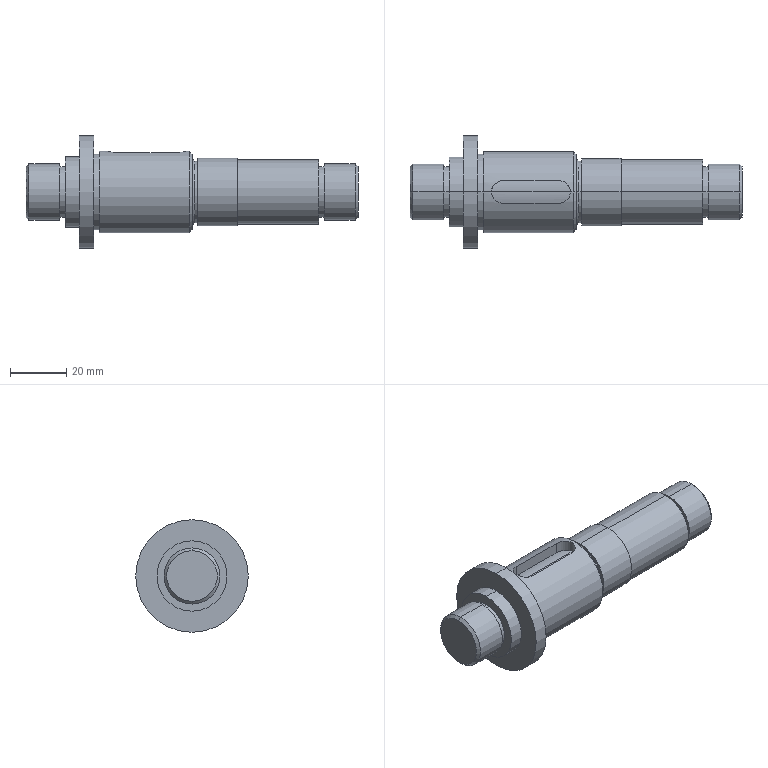Part | SolidWorks | features ICE 11, Chamfer 1, Extrusion 1 | 1 solid | 48 faces | box 118 x 40 x 40 mm | volume 58470 mm3 | cylinder 24 | plane 14 | cone 8 | spline 2 | commonest cylinder face diameters 18 x4 20 x4 29 x4 22 x2 23 x2 24 x2
STEP:
#1=CARTESIAN_POINT('',(0.,0.,9.));
#2=VERTEX_POINT('',#1);
#3=CARTESIAN_POINT('',(0.,0.,-9.));
#4=VERTEX_POINT('',#3);
#5=CARTESIAN_POINT('',(0.,0.,0.));
#6=DIRECTION('',(-1.,0.,0.));
#7=DIRECTION('',(0.,0.,-1.));
#8=AXIS2_PLACEMENT_3D('',#5,#6,#7);
#9=CIRCLE('',#8,9.);
#10=EDGE_CURVE('',#2,#4,#9,.T.);
#11=ORIENTED_EDGE('',*,*,#10,.F.);
#12=CARTESIAN_POINT('',(1.,0.,10.));
#13=VERTEX_POINT('',#12);
#14=CARTESIAN_POINT('',(1.,0.,10.));
#15=DIRECTION('',(0.7071,0.,0.7071));
#16=VECTOR('',#15,1000.);
#17=LINE('',#14,#16);
#18=EDGE_CURVE('',#2,#13,#17,.T.);
#19=ORIENTED_EDGE('',*,*,#18,.T.);
#20=CARTESIAN_POINT('',(1.,0.,-10.));
#21=VERTEX_POINT('',#20);
#22=CARTESIAN_POINT('',(1.,0.,0.));
#23=DIRECTION('',(1.,0.,0.));
#24=DIRECTION('',(0.,0.,-1.));
#25=AXIS2_PLACEMENT_3D('',#22,#23,#24);
#26=CIRCLE('',#25,10.);
#27=EDGE_CURVE('',#21,#13,#26,.T.);
#28=ORIENTED_EDGE('',*,*,#27,.F.);
#29=CARTESIAN_POINT('',(1.,0.,-10.));
#30=DIRECTION('',(0.7071,0.,-0.7071));
#31=VECTOR('',#30,1000.);
#32=LINE('',#29,#31);
#33=EDGE_CURVE('',#4,#21,#32,.T.);
#34=ORIENTED_EDGE('',*,*,#33,.F.);
#35=EDGE_LOOP('',(#11,#19,#28,#34));
#36=FACE_OUTER_BOUND('',#35,.T.);
#37=CARTESIAN_POINT('',(1.,0.,0.));
#38=DIRECTION('',(1.,0.,0.));
#39=DIRECTION('',(0.,0.,-1.));
#40=AXIS2_PLACEMENT_3D('',#37,#38,#39);
#41=CONICAL_SURFACE('',#40,10.,0.7854);
#42=ADVANCED_FACE('',(#36),#41,.T.);
#43=CARTESIAN_POINT('',(118.,0.,-9.));
#44=VERTEX_POINT('',#43);
#45=CARTESIAN_POINT('',(118.,0.,9.));
#46=VERTEX_POINT('',#45);
#47=CARTESIAN_POINT('',(118.,0.,0.));
#48=DIRECTION('',(1.,0.,0.));
#49=DIRECTION('',(0.,0.,-1.));
#50=AXIS2_PLACEMENT_3D('',#47,#48,#49);
#51=CIRCLE('',#50,9.);
#52=EDGE_CURVE('',#44,#46,#51,.T.);
#53=ORIENTED_EDGE('',*,*,#52,.F.);
#54=CARTESIAN_POINT('',(117.,0.,-10.));
#55=VERTEX_POINT('',#54);
#56=CARTESIAN_POINT('',(118.,0.,-9.));
#57=DIRECTION('',(-0.7071,0.,-0.7071));
#58=VECTOR('',#57,1000.);
#59=LINE('',#56,#58);
#60=EDGE_CURVE('',#44,#55,#59,.T.);
#61=ORIENTED_EDGE('',*,*,#60,.T.);
#62=CARTESIAN_POINT('',(117.,0.,10.));
#63=VERTEX_POINT('',#62);
#64=CARTESIAN_POINT('',(117.,0.,0.));
#65=DIRECTION('',(-1.,0.,0.));
#66=DIRECTION('',(0.,0.,-1.));
#67=AXIS2_PLACEMENT_3D('',#64,#65,#66);
#68=CIRCLE('',#67,10.);
#69=EDGE_CURVE('',#63,#55,#68,.T.);
#70=ORIENTED_EDGE('',*,*,#69,.F.);
#71=CARTESIAN_POINT('',(118.,0.,9.));
#72=DIRECTION('',(-0.7071,0.,0.7071));
#73=VECTOR('',#72,1000.);
#74=LINE('',#71,#73);
#75=EDGE_CURVE('',#46,#63,#74,.T.);
#76=ORIENTED_EDGE('',*,*,#75,.F.);
#77=EDGE_LOOP('',(#53,#61,#70,#76));
#78=FACE_OUTER_BOUND('',#77,.T.);
#79=CARTESIAN_POINT('',(118.,0.,0.));
#80=DIRECTION('',(-1.,0.,0.));
#81=DIRECTION('',(0.,0.,1.));
#82=AXIS2_PLACEMENT_3D('',#79,#80,#81);
#83=CONICAL_SURFACE('',#82,9.,0.7854);
#84=ADVANCED_FACE('',(#78),#83,.T.);
#85=CARTESIAN_POINT('',(60.,0.,-11.));
#86=VERTEX_POINT('',#85);
#87=CARTESIAN_POINT('',(60.,0.,11.));
#88=VERTEX_POINT('',#87);
#89=CARTESIAN_POINT('',(60.,0.,0.));
#90=DIRECTION('',(1.,0.,0.));
#91=DIRECTION('',(0.,0.,-1.));
#92=AXIS2_PLACEMENT_3D('',#89,#90,#91);
#93=CIRCLE('',#92,11.);
#94=EDGE_CURVE('',#86,#88,#93,.T.);
#95=ORIENTED_EDGE('',*,*,#94,.F.);
#96=CARTESIAN_POINT('',(59.,0.,-12.));
#97=VERTEX_POINT('',#96);
#98=CARTESIAN_POINT('',(60.,0.,-11.));
#99=DIRECTION('',(-0.7071,0.,-0.7071));
#100=VECTOR('',#99,1000.);
#101=LINE('',#98,#100);
#102=EDGE_CURVE('',#86,#97,#101,.T.);
#103=ORIENTED_EDGE('',*,*,#102,.T.);
#104=CARTESIAN_POINT('',(59.,0.,12.));
#105=VERTEX_POINT('',#104);
#106=CARTESIAN_POINT('',(59.,0.,0.));
#107=DIRECTION('',(-1.,0.,0.));
#108=DIRECTION('',(0.,0.,-1.));
#109=AXIS2_PLACEMENT_3D('',#106,#107,#108);
#110=CIRCLE('',#109,12.);
#111=EDGE_CURVE('',#105,#97,#110,.T.);
#112=ORIENTED_EDGE('',*,*,#111,.F.);
#113=CARTESIAN_POINT('',(60.,0.,11.));
#114=DIRECTION('',(-0.7071,0.,0.7071));
#115=VECTOR('',#114,1000.);
#116=LINE('',#113,#115);
#117=EDGE_CURVE('',#88,#105,#116,.T.);
#118=ORIENTED_EDGE('',*,*,#117,.F.);
#119=EDGE_LOOP('',(#95,#103,#112,#118));
#120=FACE_OUTER_BOUND('',#119,.T.);
#121=CARTESIAN_POINT('',(60.,0.,0.));
#122=DIRECTION('',(-1.,0.,0.));
#123=DIRECTION('',(0.,0.,1.));
#124=AXIS2_PLACEMENT_3D('',#121,#122,#123);
#125=CONICAL_SURFACE('',#124,11.,0.7854);
#126=ADVANCED_FACE('',(#120),#125,.T.);
#127=CARTESIAN_POINT('',(59.,0.,-13.5));
#128=VERTEX_POINT('',#127);
#129=CARTESIAN_POINT('',(59.,0.,13.5));
#130=VERTEX_POINT('',#129);
#131=CARTESIAN_POINT('',(59.,0.,0.));
#132=DIRECTION('',(1.,0.,0.));
#133=DIRECTION('',(0.,0.,-1.));
#134=AXIS2_PLACEMENT_3D('',#131,#132,#133);
#135=CIRCLE('',#134,13.5);
#136=EDGE_CURVE('',#128,#130,#135,.T.);
#137=ORIENTED_EDGE('',*,*,#136,.F.);
#138=CARTESIAN_POINT('',(58.,0.,-14.5));
#139=VERTEX_POINT('',#138);
#140=CARTESIAN_POINT('',(59.,0.,-13.5));
#141=DIRECTION('',(-0.7071,0.,-0.7071));
#142=VECTOR('',#141,1000.);
#143=LINE('',#140,#142);
#144=EDGE_CURVE('',#128,#139,#143,.T.);
#145=ORIENTED_EDGE('',*,*,#144,.T.);
#146=CARTESIAN_POINT('',(58.,0.,14.5));
#147=VERTEX_POINT('',#146);
#148=CARTESIAN_POINT('',(58.,0.,0.));
#149=DIRECTION('',(-1.,0.,0.));
#150=DIRECTION('',(0.,0.,-1.));
#151=AXIS2_PLACEMENT_3D('',#148,#149,#150);
#152=CIRCLE('',#151,14.5);
#153=EDGE_CURVE('',#147,#139,#152,.T.);
#154=ORIENTED_EDGE('',*,*,#153,.F.);
#155=CARTESIAN_POINT('',(59.,0.,13.5));
#156=DIRECTION('',(-0.7071,0.,0.7071));
#157=VECTOR('',#156,1000.);
#158=LINE('',#155,#157);
#159=EDGE_CURVE('',#130,#147,#158,.T.);
#160=ORIENTED_EDGE('',*,*,#159,.F.);
#161=EDGE_LOOP('',(#137,#145,#154,#160));
#162=FACE_OUTER_BOUND('',#161,.T.);
#163=CARTESIAN_POINT('',(59.,0.,0.));
#164=DIRECTION('',(-1.,0.,0.));
#165=DIRECTION('',(0.,0.,1.));
#166=AXIS2_PLACEMENT_3D('',#163,#164,#165);
#167=CONICAL_SURFACE('',#166,13.5,0.7854);
#168=ADVANCED_FACE('',(#162),#167,.T.);
#169=CARTESIAN_POINT('',(53.,-4.,9.937));
#170=VERTEX_POINT('',#169);
#171=CARTESIAN_POINT('',(57.,0.000000128,10.5));
#172=VERTEX_POINT('',#171);
#173=CARTESIAN_POINT('',(53.,-4.,9.937));
#174=CARTESIAN_POINT('',(53.264,-4.,9.937));
#175=CARTESIAN_POINT('',(53.531,-3.972,9.945));
#176=CARTESIAN_POINT('',(54.044,-3.867,9.975));
#177=CARTESIAN_POINT('',(54.297,-3.789,9.997));
#178=CARTESIAN_POINT('',(55.02,-3.488,10.076));
#179=CARTESIAN_POINT('',(55.464,-3.193,10.149));
#180=CARTESIAN_POINT('',(56.012,-2.644,10.258));
#181=CARTESIAN_POINT('',(56.178,-2.441,10.295));
#182=CARTESIAN_POINT('',(56.466,-2.006,10.362));
#183=CARTESIAN_POINT('',(56.589,-1.775,10.393));
#184=CARTESIAN_POINT('',(56.791,-1.29,10.445));
#185=CARTESIAN_POINT('',(56.868,-1.04,10.465));
#186=CARTESIAN_POINT('',(56.973,-0.5231,10.493));
#187=CARTESIAN_POINT('',(57.,-0.2611,10.5));
#188=CARTESIAN_POINT('',(57.,0.000000128,10.5));
#189=B_SPLINE_CURVE_WITH_KNOTS('',3,(#173,#174,#175,#176,#177,#178,#179,#180,#181,#182,#183,#184,#185,#186,#187,#188),.UNSPECIFIED.,.F.,.F.,(4,2,2,2,2,2,2,4),(0.,0.06254,0.1251,0.2501,0.3127,0.3752,0.4378,0.5003),.UNSPECIFIED.);
#190=EDGE_CURVE('',#170,#172,#189,.T.);
#191=ORIENTED_EDGE('',*,*,#190,.T.);
#192=CARTESIAN_POINT('',(29.,-0.000000128,10.5));
#193=VERTEX_POINT('',#192);
#194=CARTESIAN_POINT('',(59.,0.,10.5));
#195=DIRECTION('',(-1.,0.,0.));
#196=VECTOR('',#195,1000.);
#197=LINE('',#194,#196);
#198=EDGE_CURVE('',#172,#193,#197,.T.);
#199=ORIENTED_EDGE('',*,*,#198,.T.);
#200=CARTESIAN_POINT('',(33.,-4.,9.937));
#201=VERTEX_POINT('',#200);
#202=CARTESIAN_POINT('',(29.,-0.000000128,10.5));
#203=CARTESIAN_POINT('',(29.,-0.2608,10.5));
#204=CARTESIAN_POINT('',(29.027,-0.5243,10.493));
#205=CARTESIAN_POINT('',(29.131,-1.037,10.465));
#206=CARTESIAN_POINT('',(29.208,-1.288,10.445));
#207=CARTESIAN_POINT('',(29.509,-2.015,10.368));
#208=CARTESIAN_POINT('',(29.803,-2.46,10.295));
#209=CARTESIAN_POINT('',(30.356,-3.013,10.185));
#210=CARTESIAN_POINT('',(30.559,-3.179,10.148));
#211=CARTESIAN_POINT('',(30.993,-3.468,10.08));
#212=CARTESIAN_POINT('',(31.223,-3.591,10.049));
#213=CARTESIAN_POINT('',(31.707,-3.792,9.996));
#214=CARTESIAN_POINT('',(31.955,-3.868,9.975));
#215=CARTESIAN_POINT('',(32.343,-3.947,9.953));
#216=CARTESIAN_POINT('',(32.472,-3.966,9.947));
#217=CARTESIAN_POINT('',(32.736,-3.993,9.939));
#218=CARTESIAN_POINT('',(32.868,-4.,9.937));
#219=CARTESIAN_POINT('',(33.,-4.,9.937));
#220=B_SPLINE_CURVE_WITH_KNOTS('',3,(#202,#203,#204,#205,#206,#207,#208,#209,#210,#211,#212,#213,#214,#215,#216,#217,#218,#219),.UNSPECIFIED.,.F.,.F.,(4,2,2,2,2,2,2,2,4),(0.5003,0.5628,0.6252,0.7501,0.8126,0.8751,0.9375,0.9688,1.),.UNSPECIFIED.);
#221=EDGE_CURVE('',#193,#201,#220,.T.);
#222=ORIENTED_EDGE('',*,*,#221,.T.);
#223=CARTESIAN_POINT('',(59.,-4.,9.937));
#224=DIRECTION('',(-1.,0.,0.));
#225=VECTOR('',#224,1000.);
#226=LINE('',#223,#225);
#227=EDGE_CURVE('',#170,#201,#226,.T.);
#228=ORIENTED_EDGE('',*,*,#227,.F.);
#229=EDGE_LOOP('',(#191,#199,#222,#228));
#230=FACE_OUTER_BOUND('',#229,.T.);
#231=CARTESIAN_POINT('',(59.,0.,-4.));
#232=DIRECTION('',(-1.,0.,0.));
#233=DIRECTION('',(0.,0.,1.));
#234=AXIS2_PLACEMENT_3D('',#231,#232,#233);
#235=CYLINDRICAL_SURFACE('',#234,14.5);
#236=ADVANCED_FACE('',(#230),#235,.T.);
#237=ORIENTED_EDGE('',*,*,#69,.T.);
#238=CARTESIAN_POINT('',(106.,0.,-10.));
#239=VERTEX_POINT('',#238);
#240=CARTESIAN_POINT('',(118.,0.,-10.));
#241=DIRECTION('',(-1.,0.,0.));
#242=VECTOR('',#241,1000.);
#243=LINE('',#240,#242);
#244=EDGE_CURVE('',#55,#239,#243,.T.);
#245=ORIENTED_EDGE('',*,*,#244,.T.);
#246=CARTESIAN_POINT('',(106.,0.,10.));
#247=VERTEX_POINT('',#246);
#248=CARTESIAN_POINT('',(106.,0.,0.));
#249=DIRECTION('',(1.,0.,0.));
#250=DIRECTION('',(0.,0.,-1.));
#251=AXIS2_PLACEMENT_3D('',#248,#249,#250);
#252=CIRCLE('',#251,10.);
#253=EDGE_CURVE('',#239,#247,#252,.T.);
#254=ORIENTED_EDGE('',*,*,#253,.T.);
#255=CARTESIAN_POINT('',(118.,0.,10.));
#256=DIRECTION('',(-1.,0.,0.));
#257=VECTOR('',#256,1000.);
#258=LINE('',#255,#257);
#259=EDGE_CURVE('',#63,#247,#258,.T.);
#260=ORIENTED_EDGE('',*,*,#259,.F.);
#261=EDGE_LOOP('',(#237,#245,#254,#260));
#262=FACE_OUTER_BOUND('',#261,.T.);
#263=CARTESIAN_POINT('',(118.,0.,0.));
#264=DIRECTION('',(-1.,0.,0.));
#265=DIRECTION('',(0.,0.,1.));
#266=AXIS2_PLACEMENT_3D('',#263,#264,#265);
#267=CYLINDRICAL_SURFACE('',#266,10.);
#268=ADVANCED_FACE('',(#262),#267,.T.);
#269=CARTESIAN_POINT('',(106.,0.,-9.));
#270=VERTEX_POINT('',#269);
#271=CARTESIAN_POINT('',(106.,0.,9.));
#272=VERTEX_POINT('',#271);
#273=CARTESIAN_POINT('',(106.,0.,0.));
#274=DIRECTION('',(1.,0.,0.));
#275=DIRECTION('',(0.,0.,-1.));
#276=AXIS2_PLACEMENT_3D('',#273,#274,#275);
#277=CIRCLE('',#276,9.);
#278=EDGE_CURVE('',#270,#272,#277,.T.);
#279=ORIENTED_EDGE('',*,*,#278,.F.);
#280=CARTESIAN_POINT('',(104.,0.,-9.));
#281=VERTEX_POINT('',#280);
#282=CARTESIAN_POINT('',(106.,0.,-9.));
#283=DIRECTION('',(-1.,0.,0.));
#284=VECTOR('',#283,1000.);
#285=LINE('',#282,#284);
#286=EDGE_CURVE('',#270,#281,#285,.T.);
#287=ORIENTED_EDGE('',*,*,#286,.T.);
#288=CARTESIAN_POINT('',(104.,0.,9.));
#289=VERTEX_POINT('',#288);
#290=CARTESIAN_POINT('',(104.,0.,0.));
#291=DIRECTION('',(1.,0.,0.));
#292=DIRECTION('',(0.,0.,-1.));
#293=AXIS2_PLACEMENT_3D('',#290,#291,#292);
#294=CIRCLE('',#293,9.);
#295=EDGE_CURVE('',#281,#289,#294,.T.);
#296=ORIENTED_EDGE('',*,*,#295,.T.);
#297=CARTESIAN_POINT('',(106.,0.,9.));
#298=DIRECTION('',(-1.,0.,0.));
#299=VECTOR('',#298,1000.);
#300=LINE('',#297,#299);
#301=EDGE_CURVE('',#272,#289,#300,.T.);
#302=ORIENTED_EDGE('',*,*,#301,.F.);
#303=EDGE_LOOP('',(#279,#287,#296,#302));
#304=FACE_OUTER_BOUND('',#303,.T.);
#305=CARTESIAN_POINT('',(106.,0.,0.));
#306=DIRECTION('',(-1.,0.,0.));
#307=DIRECTION('',(0.,0.,1.));
#308=AXIS2_PLACEMENT_3D('',#305,#306,#307);
#309=CYLINDRICAL_SURFACE('',#308,9.);
#310=ADVANCED_FACE('',(#304),#309,.T.);
#311=CARTESIAN_POINT('',(104.,0.,-11.5));
#312=VERTEX_POINT('',#311);
#313=CARTESIAN_POINT('',(104.,0.,11.5));
#314=VERTEX_POINT('',#313);
#315=CARTESIAN_POINT('',(104.,0.,0.));
#316=DIRECTION('',(1.,0.,0.));
#317=DIRECTION('',(0.,0.,-1.));
#318=AXIS2_PLACEMENT_3D('',#315,#316,#317);
#319=CIRCLE('',#318,11.5);
#320=EDGE_CURVE('',#312,#314,#319,.T.);
#321=ORIENTED_EDGE('',*,*,#320,.F.);
#322=CARTESIAN_POINT('',(75.,0.,-11.5));
#323=VERTEX_POINT('',#322);
#324=CARTESIAN_POINT('',(104.,0.,-11.5));
#325=DIRECTION('',(-1.,0.,0.));
#326=VECTOR('',#325,1000.);
#327=LINE('',#324,#326);
#328=EDGE_CURVE('',#312,#323,#327,.T.);
#329=ORIENTED_EDGE('',*,*,#328,.T.);
#330=CARTESIAN_POINT('',(75.,0.,11.5));
#331=VERTEX_POINT('',#330);
#332=CARTESIAN_POINT('',(75.,0.,0.));
#333=DIRECTION('',(1.,0.,0.));
#334=DIRECTION('',(0.,0.,-1.));
#335=AXIS2_PLACEMENT_3D('',#332,#333,#334);
#336=CIRCLE('',#335,11.5);
#337=EDGE_CURVE('',#323,#331,#336,.T.);
#338=ORIENTED_EDGE('',*,*,#337,.T.);
#339=CARTESIAN_POINT('',(104.,0.,11.5));
#340=DIRECTION('',(-1.,0.,0.));
#341=VECTOR('',#340,1000.);
#342=LINE('',#339,#341);
#343=EDGE_CURVE('',#314,#331,#342,.T.);
#344=ORIENTED_EDGE('',*,*,#343,.F.);
#345=EDGE_LOOP('',(#321,#329,#338,#344));
#346=FACE_OUTER_BOUND('',#345,.T.);
#347=CARTESIAN_POINT('',(104.,0.,0.));
#348=DIRECTION('',(-1.,0.,0.));
#349=DIRECTION('',(0.,0.,1.));
#350=AXIS2_PLACEMENT_3D('',#347,#348,#349);
#351=CYLINDRICAL_SURFACE('',#350,11.5);
#352=ADVANCED_FACE('',(#346),#351,.T.);
#353=CARTESIAN_POINT('',(75.,0.,-12.));
#354=VERTEX_POINT('',#353);
#355=CARTESIAN_POINT('',(75.,0.,12.));
#356=VERTEX_POINT('',#355);
#357=CARTESIAN_POINT('',(75.,0.,0.));
#358=DIRECTION('',(1.,0.,0.));
#359=DIRECTION('',(0.,0.,-1.));
#360=AXIS2_PLACEMENT_3D('',#357,#358,#359);
#361=CIRCLE('',#360,12.);
#362=EDGE_CURVE('',#354,#356,#361,.T.);
#363=ORIENTED_EDGE('',*,*,#362,.F.);
#364=CARTESIAN_POINT('',(61.,0.,-12.));
#365=VERTEX_POINT('',#364);
#366=CARTESIAN_POINT('',(75.,0.,-12.));
#367=DIRECTION('',(-1.,0.,0.));
#368=VECTOR('',#367,1000.);
#369=LINE('',#366,#368);
#370=EDGE_CURVE('',#354,#365,#369,.T.);
#371=ORIENTED_EDGE('',*,*,#370,.T.);
#372=CARTESIAN_POINT('',(61.,0.,12.));
#373=VERTEX_POINT('',#372);
#374=CARTESIAN_POINT('',(61.,0.,0.));
#375=DIRECTION('',(1.,0.,0.));
#376=DIRECTION('',(0.,0.,-1.));
#377=AXIS2_PLACEMENT_3D('',#374,#375,#376);
#378=CIRCLE('',#377,12.);
#379=EDGE_CURVE('',#365,#373,#378,.T.);
#380=ORIENTED_EDGE('',*,*,#379,.T.);
#381=CARTESIAN_POINT('',(75.,0.,12.));
#382=DIRECTION('',(-1.,0.,0.));
#383=VECTOR('',#382,1000.);
#384=LINE('',#381,#383);
#385=EDGE_CURVE('',#356,#373,#384,.T.);
#386=ORIENTED_EDGE('',*,*,#385,.F.);
#387=EDGE_LOOP('',(#363,#371,#380,#386));
#388=FACE_OUTER_BOUND('',#387,.T.);
#389=CARTESIAN_POINT('',(75.,0.,0.));
#390=DIRECTION('',(-1.,0.,0.));
#391=DIRECTION('',(0.,0.,1.));
#392=AXIS2_PLACEMENT_3D('',#389,#390,#391);
#393=CYLINDRICAL_SURFACE('',#392,12.);
#394=ADVANCED_FACE('',(#388),#393,.T.);
#395=CARTESIAN_POINT('',(61.,0.,-11.));
#396=VERTEX_POINT('',#395);
#397=CARTESIAN_POINT('',(61.,0.,11.));
#398=VERTEX_POINT('',#397);
#399=CARTESIAN_POINT('',(61.,0.,0.));
#400=DIRECTION('',(1.,0.,0.));
#401=DIRECTION('',(0.,0.,-1.));
#402=AXIS2_PLACEMENT_3D('',#399,#400,#401);
#403=CIRCLE('',#402,11.);
#404=EDGE_CURVE('',#396,#398,#403,.T.);
#405=ORIENTED_EDGE('',*,*,#404,.F.);
#406=CARTESIAN_POINT('',(61.,0.,-11.));
#407=DIRECTION('',(-1.,0.,0.));
#408=VECTOR('',#407,1000.);
#409=LINE('',#406,#408);
#410=EDGE_CURVE('',#396,#86,#409,.T.);
#411=ORIENTED_EDGE('',*,*,#410,.T.);
#412=ORIENTED_EDGE('',*,*,#94,.T.);
#413=CARTESIAN_POINT('',(61.,0.,11.));
#414=DIRECTION('',(-1.,0.,0.));
#415=VECTOR('',#414,1000.);
#416=LINE('',#413,#415);
#417=EDGE_CURVE('',#398,#88,#416,.T.);
#418=ORIENTED_EDGE('',*,*,#417,.F.);
#419=EDGE_LOOP('',(#405,#411,#412,#418));
#420=FACE_OUTER_BOUND('',#419,.T.);
#421=CARTESIAN_POINT('',(61.,0.,0.));
#422=DIRECTION('',(-1.,0.,0.));
#423=DIRECTION('',(0.,0.,1.));
#424=AXIS2_PLACEMENT_3D('',#421,#422,#423);
#425=CYLINDRICAL_SURFACE('',#424,11.);
#426=ADVANCED_FACE('',(#420),#425,.T.);
#427=ORIENTED_EDGE('',*,*,#153,.T.);
#428=CARTESIAN_POINT('',(26.,0.,-14.5));
#429=VERTEX_POINT('',#428);
#430=CARTESIAN_POINT('',(59.,0.,-14.5));
#431=DIRECTION('',(-1.,0.,0.));
#432=VECTOR('',#431,1000.);
#433=LINE('',#430,#432);
#434=EDGE_CURVE('',#139,#429,#433,.T.);
#435=ORIENTED_EDGE('',*,*,#434,.T.);
#436=CARTESIAN_POINT('',(26.,0.,14.5));
#437=VERTEX_POINT('',#436);
#438=CARTESIAN_POINT('',(26.,0.,0.));
#439=DIRECTION('',(1.,0.,0.));
#440=DIRECTION('',(0.,0.,-1.));
#441=AXIS2_PLACEMENT_3D('',#438,#439,#440);
#442=CIRCLE('',#441,14.5);
#443=EDGE_CURVE('',#429,#437,#442,.T.);
#444=ORIENTED_EDGE('',*,*,#443,.T.);
#445=CARTESIAN_POINT('',(29.,0.000006792,14.5));
#446=VERTEX_POINT('',#445);
#447=CARTESIAN_POINT('',(59.,0.,14.5));
#448=DIRECTION('',(-1.,0.,0.));
#449=VECTOR('',#448,1000.);
#450=LINE('',#447,#449);
#451=EDGE_CURVE('',#446,#437,#450,.T.);
#452=ORIENTED_EDGE('',*,*,#451,.F.);
#453=CARTESIAN_POINT('',(33.,4.,13.937));
#454=VERTEX_POINT('',#453);
#455=CARTESIAN_POINT('',(33.,4.,13.937));
#456=CARTESIAN_POINT('',(31.938,4.,13.937));
#457=CARTESIAN_POINT('',(30.906,3.562,14.075));
#458=CARTESIAN_POINT('',(29.438,2.095,14.367));
#459=CARTESIAN_POINT('',(29.001,1.053,14.5));
#460=CARTESIAN_POINT('',(29.,0.002502,14.5));
#461=CARTESIAN_POINT('',(29.,0.001255,14.5));
#462=CARTESIAN_POINT('',(29.,0.000006792,14.5));
#463=B_SPLINE_CURVE_WITH_KNOTS('',3,(#455,#456,#457,#458,#459,#460,#461,#462),.UNSPECIFIED.,.F.,.F.,(4,2,2,4),(0.,0.25,0.5,0.5003),.UNSPECIFIED.);
#464=EDGE_CURVE('',#454,#446,#463,.T.);
#465=ORIENTED_EDGE('',*,*,#464,.F.);
#466=CARTESIAN_POINT('',(53.,4.,13.937));
#467=VERTEX_POINT('',#466);
#468=CARTESIAN_POINT('',(59.,4.,13.937));
#469=DIRECTION('',(-1.,0.,0.));
#470=VECTOR('',#469,1000.);
#471=LINE('',#468,#470);
#472=EDGE_CURVE('',#467,#454,#471,.T.);
#473=ORIENTED_EDGE('',*,*,#472,.F.);
#474=CARTESIAN_POINT('',(57.,-0.000006792,14.5));
#475=VERTEX_POINT('',#474);
#476=CARTESIAN_POINT('',(57.,-0.000006792,14.5));
#477=CARTESIAN_POINT('',(57.,1.048,14.5));
#478=CARTESIAN_POINT('',(56.568,2.088,14.369));
#479=CARTESIAN_POINT('',(55.09,3.567,14.075));
#480=CARTESIAN_POINT('',(54.062,4.,13.937));
#481=CARTESIAN_POINT('',(53.,4.,13.937));
#482=B_SPLINE_CURVE_WITH_KNOTS('',3,(#476,#477,#478,#479,#480,#481),.UNSPECIFIED.,.F.,.F.,(4,2,4),(0.5003,0.75,1.),.UNSPECIFIED.);
#483=EDGE_CURVE('',#475,#467,#482,.T.);
#484=ORIENTED_EDGE('',*,*,#483,.F.);
#485=CARTESIAN_POINT('',(59.,0.,14.5));
#486=DIRECTION('',(-1.,0.,0.));
#487=VECTOR('',#486,1000.);
#488=LINE('',#485,#487);
#489=EDGE_CURVE('',#147,#475,#488,.T.);
#490=ORIENTED_EDGE('',*,*,#489,.F.);
#491=EDGE_LOOP('',(#427,#435,#444,#452,#465,#473,#484,#490));
#492=FACE_OUTER_BOUND('',#491,.T.);
#493=CARTESIAN_POINT('',(59.,0.,0.));
#494=DIRECTION('',(-1.,0.,0.));
#495=DIRECTION('',(0.,0.,1.));
#496=AXIS2_PLACEMENT_3D('',#493,#494,#495);
#497=CYLINDRICAL_SURFACE('',#496,14.5);
#498=ADVANCED_FACE('',(#492),#497,.T.);
#499=CARTESIAN_POINT('',(26.,0.,-13.5));
#500=VERTEX_POINT('',#499);
#501=CARTESIAN_POINT('',(26.,0.,13.5));
#502=VERTEX_POINT('',#501);
#503=CARTESIAN_POINT('',(26.,0.,0.));
#504=DIRECTION('',(1.,0.,0.));
#505=DIRECTION('',(0.,0.,-1.));
#506=AXIS2_PLACEMENT_3D('',#503,#504,#505);
#507=CIRCLE('',#506,13.5);
#508=EDGE_CURVE('',#500,#502,#507,.T.);
#509=ORIENTED_EDGE('',*,*,#508,.F.);
#510=CARTESIAN_POINT('',(24.,0.,-13.5));
#511=VERTEX_POINT('',#510);
#512=CARTESIAN_POINT('',(26.,0.,-13.5));
#513=DIRECTION('',(-1.,0.,0.));
#514=VECTOR('',#513,1000.);
#515=LINE('',#512,#514);
#516=EDGE_CURVE('',#500,#511,#515,.T.);
#517=ORIENTED_EDGE('',*,*,#516,.T.);
#518=CARTESIAN_POINT('',(24.,0.,13.5));
#519=VERTEX_POINT('',#518);
#520=CARTESIAN_POINT('',(24.,0.,0.));
#521=DIRECTION('',(1.,0.,0.));
#522=DIRECTION('',(0.,0.,-1.));
#523=AXIS2_PLACEMENT_3D('',#520,#521,#522);
#524=CIRCLE('',#523,13.5);
#525=EDGE_CURVE('',#511,#519,#524,.T.);
#526=ORIENTED_EDGE('',*,*,#525,.T.);
#527=CARTESIAN_POINT('',(26.,0.,13.5));
#528=DIRECTION('',(-1.,0.,0.));
#529=VECTOR('',#528,1000.);
#530=LINE('',#527,#529);
#531=EDGE_CURVE('',#502,#519,#530,.T.);
#532=ORIENTED_EDGE('',*,*,#531,.F.);
#533=EDGE_LOOP('',(#509,#517,#526,#532));
#534=FACE_OUTER_BOUND('',#533,.T.);
#535=CARTESIAN_POINT('',(26.,0.,0.));
#536=DIRECTION('',(-1.,0.,0.));
#537=DIRECTION('',(0.,0.,1.));
#538=AXIS2_PLACEMENT_3D('',#535,#536,#537);
#539=CYLINDRICAL_SURFACE('',#538,13.5);
#540=ADVANCED_FACE('',(#534),#539,.T.);
#541=CARTESIAN_POINT('',(24.,0.,-20.));
#542=VERTEX_POINT('',#541);
#543=CARTESIAN_POINT('',(24.,0.,20.));
#544=VERTEX_POINT('',#543);
#545=CARTESIAN_POINT('',(24.,0.,0.));
#546=DIRECTION('',(1.,0.,0.));
#547=DIRECTION('',(0.,0.,-1.));
#548=AXIS2_PLACEMENT_3D('',#545,#546,#547);
#549=CIRCLE('',#548,20.);
#550=EDGE_CURVE('',#542,#544,#549,.T.);
#551=ORIENTED_EDGE('',*,*,#550,.F.);
#552=CARTESIAN_POINT('',(19.,0.,-20.));
#553=VERTEX_POINT('',#552);
#554=CARTESIAN_POINT('',(24.,0.,-20.));
#555=DIRECTION('',(-1.,0.,0.));
#556=VECTOR('',#555,1000.);
#557=LINE('',#554,#556);
#558=EDGE_CURVE('',#542,#553,#557,.T.);
#559=ORIENTED_EDGE('',*,*,#558,.T.);
#560=CARTESIAN_POINT('',(19.,0.,20.));
#561=VERTEX_POINT('',#560);
#562=CARTESIAN_POINT('',(19.,0.,0.));
#563=DIRECTION('',(1.,0.,0.));
#564=DIRECTION('',(0.,0.,-1.));
#565=AXIS2_PLACEMENT_3D('',#562,#563,#564);
#566=CIRCLE('',#565,20.);
#567=EDGE_CURVE('',#553,#561,#566,.T.);
#568=ORIENTED_EDGE('',*,*,#567,.T.);
#569=CARTESIAN_POINT('',(24.,0.,20.));
#570=DIRECTION('',(-1.,0.,0.));
#571=VECTOR('',#570,1000.);
#572=LINE('',#569,#571);
#573=EDGE_CURVE('',#544,#561,#572,.T.);
#574=ORIENTED_EDGE('',*,*,#573,.F.);
#575=EDGE_LOOP('',(#551,#559,#568,#574));
#576=FACE_OUTER_BOUND('',#575,.T.);
#577=CARTESIAN_POINT('',(24.,0.,0.));
#578=DIRECTION('',(-1.,0.,0.));
#579=DIRECTION('',(0.,0.,1.));
#580=AXIS2_PLACEMENT_3D('',#577,#578,#579);
#581=CYLINDRICAL_SURFACE('',#580,20.);
#582=ADVANCED_FACE('',(#576),#581,.T.);
#583=CARTESIAN_POINT('',(19.,0.,-12.5));
#584=VERTEX_POINT('',#583);
#585=CARTESIAN_POINT('',(19.,0.,12.5));
#586=VERTEX_POINT('',#585);
#587=CARTESIAN_POINT('',(19.,0.,0.));
#588=DIRECTION('',(1.,0.,0.));
#589=DIRECTION('',(0.,0.,-1.));
#590=AXIS2_PLACEMENT_3D('',#587,#588,#589);
#591=CIRCLE('',#590,12.5);
#592=EDGE_CURVE('',#584,#586,#591,.T.);
#593=ORIENTED_EDGE('',*,*,#592,.F.);
#594=CARTESIAN_POINT('',(14.,0.,-12.5));
#595=VERTEX_POINT('',#594);
#596=CARTESIAN_POINT('',(19.,0.,-12.5));
#597=DIRECTION('',(-1.,0.,0.));
#598=VECTOR('',#597,1000.);
#599=LINE('',#596,#598);
#600=EDGE_CURVE('',#584,#595,#599,.T.);
#601=ORIENTED_EDGE('',*,*,#600,.T.);
#602=CARTESIAN_POINT('',(14.,0.,12.5));
#603=VERTEX_POINT('',#602);
#604=CARTESIAN_POINT('',(14.,0.,0.));
#605=DIRECTION('',(1.,0.,0.));
#606=DIRECTION('',(0.,0.,-1.));
#607=AXIS2_PLACEMENT_3D('',#604,#605,#606);
#608=CIRCLE('',#607,12.5);
#609=EDGE_CURVE('',#595,#603,#608,.T.);
#610=ORIENTED_EDGE('',*,*,#609,.T.);
#611=CARTESIAN_POINT('',(19.,0.,12.5));
#612=DIRECTION('',(-1.,0.,0.));
#613=VECTOR('',#612,1000.);
#614=LINE('',#611,#613);
#615=EDGE_CURVE('',#586,#603,#614,.T.);
#616=ORIENTED_EDGE('',*,*,#615,.F.);
#617=EDGE_LOOP('',(#593,#601,#610,#616));
#618=FACE_OUTER_BOUND('',#617,.T.);
#619=CARTESIAN_POINT('',(19.,0.,0.));
#620=DIRECTION('',(-1.,0.,0.));
#621=DIRECTION('',(0.,0.,1.));
#622=AXIS2_PLACEMENT_3D('',#619,#620,#621);
#623=CYLINDRICAL_SURFACE('',#622,12.5);
#624=ADVANCED_FACE('',(#618),#623,.T.);
#625=CARTESIAN_POINT('',(14.,0.,-9.));
#626=VERTEX_POINT('',#625);
#627=CARTESIAN_POINT('',(14.,0.,9.));
#628=VERTEX_POINT('',#627);
#629=CARTESIAN_POINT('',(14.,0.,0.));
#630=DIRECTION('',(1.,0.,0.));
#631=DIRECTION('',(0.,0.,-1.));
#632=AXIS2_PLACEMENT_3D('',#629,#630,#631);
#633=CIRCLE('',#632,9.);
#634=EDGE_CURVE('',#626,#628,#633,.T.);
#635=ORIENTED_EDGE('',*,*,#634,.F.);
#636=CARTESIAN_POINT('',(12.,0.,-9.));
#637=VERTEX_POINT('',#636);
#638=CARTESIAN_POINT('',(14.,0.,-9.));
#639=DIRECTION('',(-1.,0.,0.));
#640=VECTOR('',#639,1000.);
#641=LINE('',#638,#640);
#642=EDGE_CURVE('',#626,#637,#641,.T.);
#643=ORIENTED_EDGE('',*,*,#642,.T.);
#644=CARTESIAN_POINT('',(12.,0.,9.));
#645=VERTEX_POINT('',#644);
#646=CARTESIAN_POINT('',(12.,0.,0.));
#647=DIRECTION('',(1.,0.,0.));
#648=DIRECTION('',(0.,0.,-1.));
#649=AXIS2_PLACEMENT_3D('',#646,#647,#648);
#650=CIRCLE('',#649,9.);
#651=EDGE_CURVE('',#637,#645,#650,.T.);
#652=ORIENTED_EDGE('',*,*,#651,.T.);
#653=CARTESIAN_POINT('',(14.,0.,9.));
#654=DIRECTION('',(-1.,0.,0.));
#655=VECTOR('',#654,1000.);
#656=LINE('',#653,#655);
#657=EDGE_CURVE('',#628,#645,#656,.T.);
#658=ORIENTED_EDGE('',*,*,#657,.F.);
#659=EDGE_LOOP('',(#635,#643,#652,#658));
#660=FACE_OUTER_BOUND('',#659,.T.);
#661=CARTESIAN_POINT('',(14.,0.,0.));
#662=DIRECTION('',(-1.,0.,0.));
#663=DIRECTION('',(0.,0.,1.));
#664=AXIS2_PLACEMENT_3D('',#661,#662,#663);
#665=CYLINDRICAL_SURFACE('',#664,9.);
#666=ADVANCED_FACE('',(#660),#665,.T.);
#667=CARTESIAN_POINT('',(12.,0.,-10.));
#668=VERTEX_POINT('',#667);
#669=CARTESIAN_POINT('',(12.,0.,10.));
#670=VERTEX_POINT('',#669);
#671=CARTESIAN_POINT('',(12.,0.,0.));
#672=DIRECTION('',(1.,0.,0.));
#673=DIRECTION('',(0.,0.,-1.));
#674=AXIS2_PLACEMENT_3D('',#671,#672,#673);
#675=CIRCLE('',#674,10.);
#676=EDGE_CURVE('',#668,#670,#675,.T.);
#677=ORIENTED_EDGE('',*,*,#676,.F.);
#678=CARTESIAN_POINT('',(12.,0.,-10.));
#679=DIRECTION('',(-1.,0.,0.));
#680=VECTOR('',#679,1000.);
#681=LINE('',#678,#680);
#682=EDGE_CURVE('',#668,#21,#681,.T.);
#683=ORIENTED_EDGE('',*,*,#682,.T.);
#684=ORIENTED_EDGE('',*,*,#27,.T.);
#685=CARTESIAN_POINT('',(12.,0.,10.));
#686=DIRECTION('',(-1.,0.,0.));
#687=VECTOR('',#686,1000.);
#688=LINE('',#685,#687);
#689=EDGE_CURVE('',#670,#13,#688,.T.);
#690=ORIENTED_EDGE('',*,*,#689,.F.);
#691=EDGE_LOOP('',(#677,#683,#684,#690));
#692=FACE_OUTER_BOUND('',#691,.T.);
#693=CARTESIAN_POINT('',(12.,0.,0.));
#694=DIRECTION('',(-1.,0.,0.));
#695=DIRECTION('',(0.,0.,1.));
#696=AXIS2_PLACEMENT_3D('',#693,#694,#695);
#697=CYLINDRICAL_SURFACE('',#696,10.);
#698=ADVANCED_FACE('',(#692),#697,.T.);
#699=ORIENTED_EDGE('',*,*,#682,.F.);
#700=CARTESIAN_POINT('',(12.,0.,0.));
#701=DIRECTION('',(1.,0.,0.));
#702=DIRECTION('',(0.,0.,-1.));
#703=AXIS2_PLACEMENT_3D('',#700,#701,#702);
#704=CIRCLE('',#703,10.);
#705=EDGE_CURVE('',#670,#668,#704,.T.);
#706=ORIENTED_EDGE('',*,*,#705,.F.);
#707=ORIENTED_EDGE('',*,*,#689,.T.);
#708=CARTESIAN_POINT('',(1.,0.,0.));
#709=DIRECTION('',(1.,0.,0.));
#710=DIRECTION('',(0.,0.,-1.));
#711=AXIS2_PLACEMENT_3D('',#708,#709,#710);
#712=CIRCLE('',#711,10.);
#713=EDGE_CURVE('',#13,#21,#712,.T.);
#714=ORIENTED_EDGE('',*,*,#713,.T.);
#715=EDGE_LOOP('',(#699,#706,#707,#714));
#716=FACE_OUTER_BOUND('',#715,.T.);
#717=CARTESIAN_POINT('',(12.,0.,0.));
#718=DIRECTION('',(-1.,0.,0.));
#719=DIRECTION('',(0.,0.,1.));
#720=AXIS2_PLACEMENT_3D('',#717,#718,#719);
#721=CYLINDRICAL_SURFACE('',#720,10.);
#722=ADVANCED_FACE('',(#716),#721,.T.);
#723=CARTESIAN_POINT('',(12.,0.,0.));
#724=DIRECTION('',(1.,0.,0.));
#725=DIRECTION('',(0.,0.,-1.));
#726=AXIS2_PLACEMENT_3D('',#723,#724,#725);
#727=CIRCLE('',#726,9.);
#728=EDGE_CURVE('',#645,#637,#727,.T.);
#729=ORIENTED_EDGE('',*,*,#728,.F.);
#730=ORIENTED_EDGE('',*,*,#651,.F.);
#731=EDGE_LOOP('',(#729,#730));
#732=FACE_BOUND('',#731,.T.);
#733=ORIENTED_EDGE('',*,*,#705,.T.);
#734=ORIENTED_EDGE('',*,*,#676,.T.);
#735=EDGE_LOOP('',(#733,#734));
#736=FACE_OUTER_BOUND('',#735,.T.);
#737=CARTESIAN_POINT('',(12.,0.,0.));
#738=DIRECTION('',(1.,0.,0.));
#739=DIRECTION('',(0.,0.,-1.));
#740=AXIS2_PLACEMENT_3D('',#737,#738,#739);
#741=PLANE('',#740);
#742=ADVANCED_FACE('',(#732,#736),#741,.T.);
#743=CARTESIAN_POINT('',(0.,0.,0.));
#744=DIRECTION('',(-1.,0.,0.));
#745=DIRECTION('',(0.,0.,-1.));
#746=AXIS2_PLACEMENT_3D('',#743,#744,#745);
#747=CIRCLE('',#746,9.);
#748=EDGE_CURVE('',#4,#2,#747,.T.);
#749=ORIENTED_EDGE('',*,*,#748,.T.);
#750=ORIENTED_EDGE('',*,*,#10,.T.);
#751=EDGE_LOOP('',(#749,#750));
#752=FACE_OUTER_BOUND('',#751,.T.);
#753=CARTESIAN_POINT('',(0.,0.,0.));
#754=DIRECTION('',(1.,0.,0.));
#755=DIRECTION('',(0.,0.,-1.));
#756=AXIS2_PLACEMENT_3D('',#753,#754,#755);
#757=PLANE('',#756);
#758=ADVANCED_FACE('',(#752),#757,.F.);
#759=ORIENTED_EDGE('',*,*,#642,.F.);
#760=CARTESIAN_POINT('',(14.,0.,0.));
#761=DIRECTION('',(1.,0.,0.));
#762=DIRECTION('',(0.,0.,-1.));
#763=AXIS2_PLACEMENT_3D('',#760,#761,#762);
#764=CIRCLE('',#763,9.);
#765=EDGE_CURVE('',#628,#626,#764,.T.);
#766=ORIENTED_EDGE('',*,*,#765,.F.);
#767=ORIENTED_EDGE('',*,*,#657,.T.);
#768=ORIENTED_EDGE('',*,*,#728,.T.);
#769=EDGE_LOOP('',(#759,#766,#767,#768));
#770=FACE_OUTER_BOUND('',#769,.T.);
#771=CARTESIAN_POINT('',(14.,0.,0.));
#772=DIRECTION('',(-1.,0.,0.));
#773=DIRECTION('',(0.,0.,1.));
#774=AXIS2_PLACEMENT_3D('',#771,#772,#773);
#775=CYLINDRICAL_SURFACE('',#774,9.);
#776=ADVANCED_FACE('',(#770),#775,.T.);
#777=ORIENTED_EDGE('',*,*,#600,.F.);
#778=CARTESIAN_POINT('',(19.,0.,0.));
#779=DIRECTION('',(1.,0.,0.));
#780=DIRECTION('',(0.,0.,-1.));
#781=AXIS2_PLACEMENT_3D('',#778,#779,#780);
#782=CIRCLE('',#781,12.5);
#783=EDGE_CURVE('',#586,#584,#782,.T.);
#784=ORIENTED_EDGE('',*,*,#783,.F.);
#785=ORIENTED_EDGE('',*,*,#615,.T.);
#786=CARTESIAN_POINT('',(14.,0.,0.));
#787=DIRECTION('',(1.,0.,0.));
#788=DIRECTION('',(0.,0.,-1.));
#789=AXIS2_PLACEMENT_3D('',#786,#787,#788);
#790=CIRCLE('',#789,12.5);
#791=EDGE_CURVE('',#603,#595,#790,.T.);
#792=ORIENTED_EDGE('',*,*,#791,.T.);
#793=EDGE_LOOP('',(#777,#784,#785,#792));
#794=FACE_OUTER_BOUND('',#793,.T.);
#795=CARTESIAN_POINT('',(19.,0.,0.));
#796=DIRECTION('',(-1.,0.,0.));
#797=DIRECTION('',(0.,0.,1.));
#798=AXIS2_PLACEMENT_3D('',#795,#796,#797);
#799=CYLINDRICAL_SURFACE('',#798,12.5);
#800=ADVANCED_FACE('',(#794),#799,.T.);
#801=ORIENTED_EDGE('',*,*,#765,.T.);
#802=ORIENTED_EDGE('',*,*,#634,.T.);
#803=EDGE_LOOP('',(#801,#802));
#804=FACE_BOUND('',#803,.T.);
#805=ORIENTED_EDGE('',*,*,#791,.F.);
#806=ORIENTED_EDGE('',*,*,#609,.F.);
#807=EDGE_LOOP('',(#805,#806));
#808=FACE_OUTER_BOUND('',#807,.T.);
#809=CARTESIAN_POINT('',(14.,0.,0.));
#810=DIRECTION('',(1.,0.,0.));
#811=DIRECTION('',(0.,0.,-1.));
#812=AXIS2_PLACEMENT_3D('',#809,#810,#811);
#813=PLANE('',#812);
#814=ADVANCED_FACE('',(#804,#808),#813,.F.);
#815=ORIENTED_EDGE('',*,*,#558,.F.);
#816=CARTESIAN_POINT('',(24.,0.,0.));
#817=DIRECTION('',(1.,0.,0.));
#818=DIRECTION('',(0.,0.,-1.));
#819=AXIS2_PLACEMENT_3D('',#816,#817,#818);
#820=CIRCLE('',#819,20.);
#821=EDGE_CURVE('',#544,#542,#820,.T.);
#822=ORIENTED_EDGE('',*,*,#821,.F.);
#823=ORIENTED_EDGE('',*,*,#573,.T.);
#824=CARTESIAN_POINT('',(19.,0.,0.));
#825=DIRECTION('',(1.,0.,0.));
#826=DIRECTION('',(0.,0.,-1.));
#827=AXIS2_PLACEMENT_3D('',#824,#825,#826);
#828=CIRCLE('',#827,20.);
#829=EDGE_CURVE('',#561,#553,#828,.T.);
#830=ORIENTED_EDGE('',*,*,#829,.T.);
#831=EDGE_LOOP('',(#815,#822,#823,#830));
#832=FACE_OUTER_BOUND('',#831,.T.);
#833=CARTESIAN_POINT('',(24.,0.,0.));
#834=DIRECTION('',(-1.,0.,0.));
#835=DIRECTION('',(0.,0.,1.));
#836=AXIS2_PLACEMENT_3D('',#833,#834,#835);
#837=CYLINDRICAL_SURFACE('',#836,20.);
#838=ADVANCED_FACE('',(#832),#837,.T.);
#839=CARTESIAN_POINT('',(24.,0.,0.));
#840=DIRECTION('',(1.,0.,0.));
#841=DIRECTION('',(0.,0.,-1.));
#842=AXIS2_PLACEMENT_3D('',#839,#840,#841);
#843=CIRCLE('',#842,13.5);
#844=EDGE_CURVE('',#519,#511,#843,.T.);
#845=ORIENTED_EDGE('',*,*,#844,.F.);
#846=ORIENTED_EDGE('',*,*,#525,.F.);
#847=EDGE_LOOP('',(#845,#846));
#848=FACE_BOUND('',#847,.T.);
#849=ORIENTED_EDGE('',*,*,#821,.T.);
#850=ORIENTED_EDGE('',*,*,#550,.T.);
#851=EDGE_LOOP('',(#849,#850));
#852=FACE_OUTER_BOUND('',#851,.T.);
#853=CARTESIAN_POINT('',(24.,0.,0.));
#854=DIRECTION('',(1.,0.,0.));
#855=DIRECTION('',(0.,0.,-1.));
#856=AXIS2_PLACEMENT_3D('',#853,#854,#855);
#857=PLANE('',#856);
#858=ADVANCED_FACE('',(#848,#852),#857,.T.);
#859=ORIENTED_EDGE('',*,*,#783,.T.);
#860=ORIENTED_EDGE('',*,*,#592,.T.);
#861=EDGE_LOOP('',(#859,#860));
#862=FACE_BOUND('',#861,.T.);
#863=ORIENTED_EDGE('',*,*,#829,.F.);
#864=ORIENTED_EDGE('',*,*,#567,.F.);
#865=EDGE_LOOP('',(#863,#864));
#866=FACE_OUTER_BOUND('',#865,.T.);
#867=CARTESIAN_POINT('',(19.,0.,0.));
#868=DIRECTION('',(1.,0.,0.));
#869=DIRECTION('',(0.,0.,-1.));
#870=AXIS2_PLACEMENT_3D('',#867,#868,#869);
#871=PLANE('',#870);
#872=ADVANCED_FACE('',(#862,#866),#871,.F.);
#873=ORIENTED_EDGE('',*,*,#516,.F.);
#874=CARTESIAN_POINT('',(26.,0.,0.));
#875=DIRECTION('',(1.,0.,0.));
#876=DIRECTION('',(0.,0.,-1.));
#877=AXIS2_PLACEMENT_3D('',#874,#875,#876);
#878=CIRCLE('',#877,13.5);
#879=EDGE_CURVE('',#502,#500,#878,.T.);
#880=ORIENTED_EDGE('',*,*,#879,.F.);
#881=ORIENTED_EDGE('',*,*,#531,.T.);
#882=ORIENTED_EDGE('',*,*,#844,.T.);
#883=EDGE_LOOP('',(#873,#880,#881,#882));
#884=FACE_OUTER_BOUND('',#883,.T.);
#885=CARTESIAN_POINT('',(26.,0.,0.));
#886=DIRECTION('',(-1.,0.,0.));
#887=DIRECTION('',(0.,0.,1.));
#888=AXIS2_PLACEMENT_3D('',#885,#886,#887);
#889=CYLINDRICAL_SURFACE('',#888,13.5);
#890=ADVANCED_FACE('',(#884),#889,.T.);
#891=ORIENTED_EDGE('',*,*,#434,.F.);
#892=CARTESIAN_POINT('',(58.,0.,0.));
#893=DIRECTION('',(-1.,0.,0.));
#894=DIRECTION('',(0.,0.,-1.));
#895=AXIS2_PLACEMENT_3D('',#892,#893,#894);
#896=CIRCLE('',#895,14.5);
#897=EDGE_CURVE('',#139,#147,#896,.T.);
#898=ORIENTED_EDGE('',*,*,#897,.T.);
#899=ORIENTED_EDGE('',*,*,#489,.T.);
#900=CARTESIAN_POINT('',(53.,-4.,13.937));
#901=VERTEX_POINT('',#900);
#902=CARTESIAN_POINT('',(53.,-4.,13.937));
#903=CARTESIAN_POINT('',(54.062,-4.,13.937));
#904=CARTESIAN_POINT('',(55.094,-3.562,14.075));
#905=CARTESIAN_POINT('',(56.562,-2.095,14.367));
#906=CARTESIAN_POINT('',(56.999,-1.053,14.5));
#907=CARTESIAN_POINT('',(57.,-0.002502,14.5));
#908=CARTESIAN_POINT('',(57.,-0.001255,14.5));
#909=CARTESIAN_POINT('',(57.,-0.000006792,14.5));
#910=B_SPLINE_CURVE_WITH_KNOTS('',3,(#902,#903,#904,#905,#906,#907,#908,#909),.UNSPECIFIED.,.F.,.F.,(4,2,2,4),(0.,0.25,0.5,0.5003),.UNSPECIFIED.);
#911=EDGE_CURVE('',#901,#475,#910,.T.);
#912=ORIENTED_EDGE('',*,*,#911,.F.);
#913=CARTESIAN_POINT('',(33.,-4.,13.937));
#914=VERTEX_POINT('',#913);
#915=CARTESIAN_POINT('',(59.,-4.,13.937));
#916=DIRECTION('',(-1.,0.,0.));
#917=VECTOR('',#916,1000.);
#918=LINE('',#915,#917);
#919=EDGE_CURVE('',#901,#914,#918,.T.);
#920=ORIENTED_EDGE('',*,*,#919,.T.);
#921=CARTESIAN_POINT('',(29.,0.000006792,14.5));
#922=CARTESIAN_POINT('',(29.,-1.048,14.5));
#923=CARTESIAN_POINT('',(29.432,-2.088,14.369));
#924=CARTESIAN_POINT('',(30.91,-3.567,14.075));
#925=CARTESIAN_POINT('',(31.938,-4.,13.937));
#926=CARTESIAN_POINT('',(33.,-4.,13.937));
#927=B_SPLINE_CURVE_WITH_KNOTS('',3,(#921,#922,#923,#924,#925,#926),.UNSPECIFIED.,.F.,.F.,(4,2,4),(0.5003,0.75,1.),.UNSPECIFIED.);
#928=EDGE_CURVE('',#446,#914,#927,.T.);
#929=ORIENTED_EDGE('',*,*,#928,.F.);
#930=ORIENTED_EDGE('',*,*,#451,.T.);
#931=CARTESIAN_POINT('',(26.,0.,0.));
#932=DIRECTION('',(1.,0.,0.));
#933=DIRECTION('',(0.,0.,-1.));
#934=AXIS2_PLACEMENT_3D('',#931,#932,#933);
#935=CIRCLE('',#934,14.5);
#936=EDGE_CURVE('',#437,#429,#935,.T.);
#937=ORIENTED_EDGE('',*,*,#936,.T.);
#938=EDGE_LOOP('',(#891,#898,#899,#912,#920,#929,#930,#937));
#939=FACE_OUTER_BOUND('',#938,.T.);
#940=CARTESIAN_POINT('',(59.,0.,0.));
#941=DIRECTION('',(-1.,0.,0.));
#942=DIRECTION('',(0.,0.,1.));
#943=AXIS2_PLACEMENT_3D('',#940,#941,#942);
#944=CYLINDRICAL_SURFACE('',#943,14.5);
#945=ADVANCED_FACE('',(#939),#944,.T.);
#946=CARTESIAN_POINT('',(59.,0.,0.));
#947=DIRECTION('',(1.,0.,0.));
#948=DIRECTION('',(0.,0.,-1.));
#949=AXIS2_PLACEMENT_3D('',#946,#947,#948);
#950=CIRCLE('',#949,13.5);
#951=EDGE_CURVE('',#130,#128,#950,.T.);
#952=ORIENTED_EDGE('',*,*,#951,.T.);
#953=ORIENTED_EDGE('',*,*,#136,.T.);
#954=EDGE_LOOP('',(#952,#953));
#955=FACE_OUTER_BOUND('',#954,.T.);
#956=ORIENTED_EDGE('',*,*,#111,.T.);
#957=CARTESIAN_POINT('',(59.,0.,0.));
#958=DIRECTION('',(-1.,0.,0.));
#959=DIRECTION('',(0.,0.,-1.));
#960=AXIS2_PLACEMENT_3D('',#957,#958,#959);
#961=CIRCLE('',#960,12.);
#962=EDGE_CURVE('',#97,#105,#961,.T.);
#963=ORIENTED_EDGE('',*,*,#962,.T.);
#964=EDGE_LOOP('',(#956,#963));
#965=FACE_BOUND('',#964,.T.);
#966=CARTESIAN_POINT('',(59.,0.,0.));
#967=DIRECTION('',(1.,0.,0.));
#968=DIRECTION('',(0.,0.,-1.));
#969=AXIS2_PLACEMENT_3D('',#966,#967,#968);
#970=PLANE('',#969);
#971=ADVANCED_FACE('',(#955,#965),#970,.T.);
#972=ORIENTED_EDGE('',*,*,#879,.T.);
#973=ORIENTED_EDGE('',*,*,#508,.T.);
#974=EDGE_LOOP('',(#972,#973));
#975=FACE_BOUND('',#974,.T.);
#976=ORIENTED_EDGE('',*,*,#936,.F.);
#977=ORIENTED_EDGE('',*,*,#443,.F.);
#978=EDGE_LOOP('',(#976,#977));
#979=FACE_OUTER_BOUND('',#978,.T.);
#980=CARTESIAN_POINT('',(26.,0.,0.));
#981=DIRECTION('',(1.,0.,0.));
#982=DIRECTION('',(0.,0.,-1.));
#983=AXIS2_PLACEMENT_3D('',#980,#981,#982);
#984=PLANE('',#983);
#985=ADVANCED_FACE('',(#975,#979),#984,.F.);
#986=ORIENTED_EDGE('',*,*,#410,.F.);
#987=CARTESIAN_POINT('',(61.,0.,0.));
#988=DIRECTION('',(1.,0.,0.));
#989=DIRECTION('',(0.,0.,-1.));
#990=AXIS2_PLACEMENT_3D('',#987,#988,#989);
#991=CIRCLE('',#990,11.);
#992=EDGE_CURVE('',#398,#396,#991,.T.);
#993=ORIENTED_EDGE('',*,*,#992,.F.);
#994=ORIENTED_EDGE('',*,*,#417,.T.);
#995=CARTESIAN_POINT('',(60.,0.,0.));
#996=DIRECTION('',(1.,0.,0.));
#997=DIRECTION('',(0.,0.,-1.));
#998=AXIS2_PLACEMENT_3D('',#995,#996,#997);
#999=CIRCLE('',#998,11.);
#1000=EDGE_CURVE('',#88,#86,#999,.T.);
#1001=ORIENTED_EDGE('',*,*,#1000,.T.);
#1002=EDGE_LOOP('',(#986,#993,#994,#1001));
#1003=FACE_OUTER_BOUND('',#1002,.T.);
#1004=CARTESIAN_POINT('',(61.,0.,0.));
#1005=DIRECTION('',(-1.,0.,0.));
#1006=DIRECTION('',(0.,0.,1.));
#1007=AXIS2_PLACEMENT_3D('',#1004,#1005,#1006);
#1008=CYLINDRICAL_SURFACE('',#1007,11.);
#1009=ADVANCED_FACE('',(#1003),#1008,.T.);
#1010=ORIENTED_EDGE('',*,*,#370,.F.);
#1011=CARTESIAN_POINT('',(75.,0.,0.));
#1012=DIRECTION('',(1.,0.,0.));
#1013=DIRECTION('',(0.,0.,-1.));
#1014=AXIS2_PLACEMENT_3D('',#1011,#1012,#1013);
#1015=CIRCLE('',#1014,12.);
#1016=EDGE_CURVE('',#356,#354,#1015,.T.);
#1017=ORIENTED_EDGE('',*,*,#1016,.F.);
#1018=ORIENTED_EDGE('',*,*,#385,.T.);
#1019=CARTESIAN_POINT('',(61.,0.,0.));
#1020=DIRECTION('',(1.,0.,0.));
#1021=DIRECTION('',(0.,0.,-1.));
#1022=AXIS2_PLACEMENT_3D('',#1019,#1020,#1021);
#1023=CIRCLE('',#1022,12.);
#1024=EDGE_CURVE('',#373,#365,#1023,.T.);
#1025=ORIENTED_EDGE('',*,*,#1024,.T.);
#1026=EDGE_LOOP('',(#1010,#1017,#1018,#1025));
#1027=FACE_OUTER_BOUND('',#1026,.T.);
#1028=CARTESIAN_POINT('',(75.,0.,0.));
#1029=DIRECTION('',(-1.,0.,0.));
#1030=DIRECTION('',(0.,0.,1.));
#1031=AXIS2_PLACEMENT_3D('',#1028,#1029,#1030);
#1032=CYLINDRICAL_SURFACE('',#1031,12.);
#1033=ADVANCED_FACE('',(#1027),#1032,.T.);
#1034=CARTESIAN_POINT('',(75.,0.,0.));
#1035=DIRECTION('',(1.,0.,0.));
#1036=DIRECTION('',(0.,0.,-1.));
#1037=AXIS2_PLACEMENT_3D('',#1034,#1035,#1036);
#1038=CIRCLE('',#1037,11.5);
#1039=EDGE_CURVE('',#331,#323,#1038,.T.);
#1040=ORIENTED_EDGE('',*,*,#1039,.F.);
#1041=ORIENTED_EDGE('',*,*,#337,.F.);
#1042=EDGE_LOOP('',(#1040,#1041));
#1043=FACE_BOUND('',#1042,.T.);
#1044=ORIENTED_EDGE('',*,*,#1016,.T.);
#1045=ORIENTED_EDGE('',*,*,#362,.T.);
#1046=EDGE_LOOP('',(#1044,#1045));
#1047=FACE_OUTER_BOUND('',#1046,.T.);
#1048=CARTESIAN_POINT('',(75.,0.,0.));
#1049=DIRECTION('',(1.,0.,0.));
#1050=DIRECTION('',(0.,0.,-1.));
#1051=AXIS2_PLACEMENT_3D('',#1048,#1049,#1050);
#1052=PLANE('',#1051);
#1053=ADVANCED_FACE('',(#1043,#1047),#1052,.T.);
#1054=ORIENTED_EDGE('',*,*,#992,.T.);
#1055=ORIENTED_EDGE('',*,*,#404,.T.);
#1056=EDGE_LOOP('',(#1054,#1055));
#1057=FACE_BOUND('',#1056,.T.);
#1058=ORIENTED_EDGE('',*,*,#1024,.F.);
#1059=ORIENTED_EDGE('',*,*,#379,.F.);
#1060=EDGE_LOOP('',(#1058,#1059));
#1061=FACE_OUTER_BOUND('',#1060,.T.);
#1062=CARTESIAN_POINT('',(61.,0.,0.));
#1063=DIRECTION('',(1.,0.,0.));
#1064=DIRECTION('',(0.,0.,-1.));
#1065=AXIS2_PLACEMENT_3D('',#1062,#1063,#1064);
#1066=PLANE('',#1065);
#1067=ADVANCED_FACE('',(#1057,#1061),#1066,.F.);
#1068=ORIENTED_EDGE('',*,*,#328,.F.);
#1069=CARTESIAN_POINT('',(104.,0.,0.));
#1070=DIRECTION('',(1.,0.,0.));
#1071=DIRECTION('',(0.,0.,-1.));
#1072=AXIS2_PLACEMENT_3D('',#1069,#1070,#1071);
#1073=CIRCLE('',#1072,11.5);
#1074=EDGE_CURVE('',#314,#312,#1073,.T.);
#1075=ORIENTED_EDGE('',*,*,#1074,.F.);
#1076=ORIENTED_EDGE('',*,*,#343,.T.);
#1077=ORIENTED_EDGE('',*,*,#1039,.T.);
#1078=EDGE_LOOP('',(#1068,#1075,#1076,#1077));
#1079=FACE_OUTER_BOUND('',#1078,.T.);
#1080=CARTESIAN_POINT('',(104.,0.,0.));
#1081=DIRECTION('',(-1.,0.,0.));
#1082=DIRECTION('',(0.,0.,1.));
#1083=AXIS2_PLACEMENT_3D('',#1080,#1081,#1082);
#1084=CYLINDRICAL_SURFACE('',#1083,11.5);
#1085=ADVANCED_FACE('',(#1079),#1084,.T.);
#1086=CARTESIAN_POINT('',(104.,0.,0.));
#1087=DIRECTION('',(1.,0.,0.));
#1088=DIRECTION('',(0.,0.,-1.));
#1089=AXIS2_PLACEMENT_3D('',#1086,#1087,#1088);
#1090=CIRCLE('',#1089,9.);
#1091=EDGE_CURVE('',#289,#281,#1090,.T.);
#1092=ORIENTED_EDGE('',*,*,#1091,.F.);
#1093=ORIENTED_EDGE('',*,*,#295,.F.);
#1094=EDGE_LOOP('',(#1092,#1093));
#1095=FACE_BOUND('',#1094,.T.);
#1096=ORIENTED_EDGE('',*,*,#1074,.T.);
#1097=ORIENTED_EDGE('',*,*,#320,.T.);
#1098=EDGE_LOOP('',(#1096,#1097));
#1099=FACE_OUTER_BOUND('',#1098,.T.);
#1100=CARTESIAN_POINT('',(104.,0.,0.));
#1101=DIRECTION('',(1.,0.,0.));
#1102=DIRECTION('',(0.,0.,-1.));
#1103=AXIS2_PLACEMENT_3D('',#1100,#1101,#1102);
#1104=PLANE('',#1103);
#1105=ADVANCED_FACE('',(#1095,#1099),#1104,.T.);
#1106=ORIENTED_EDGE('',*,*,#286,.F.);
#1107=CARTESIAN_POINT('',(106.,0.,0.));
#1108=DIRECTION('',(1.,0.,0.));
#1109=DIRECTION('',(0.,0.,-1.));
#1110=AXIS2_PLACEMENT_3D('',#1107,#1108,#1109);
#1111=CIRCLE('',#1110,9.);
#1112=EDGE_CURVE('',#272,#270,#1111,.T.);
#1113=ORIENTED_EDGE('',*,*,#1112,.F.);
#1114=ORIENTED_EDGE('',*,*,#301,.T.);
#1115=ORIENTED_EDGE('',*,*,#1091,.T.);
#1116=EDGE_LOOP('',(#1106,#1113,#1114,#1115));
#1117=FACE_OUTER_BOUND('',#1116,.T.);
#1118=CARTESIAN_POINT('',(106.,0.,0.));
#1119=DIRECTION('',(-1.,0.,0.));
#1120=DIRECTION('',(0.,0.,1.));
#1121=AXIS2_PLACEMENT_3D('',#1118,#1119,#1120);
#1122=CYLINDRICAL_SURFACE('',#1121,9.);
#1123=ADVANCED_FACE('',(#1117),#1122,.T.);
#1124=ORIENTED_EDGE('',*,*,#244,.F.);
#1125=CARTESIAN_POINT('',(117.,0.,0.));
#1126=DIRECTION('',(-1.,0.,0.));
#1127=DIRECTION('',(0.,0.,-1.));
#1128=AXIS2_PLACEMENT_3D('',#1125,#1126,#1127);
#1129=CIRCLE('',#1128,10.);
#1130=EDGE_CURVE('',#55,#63,#1129,.T.);
#1131=ORIENTED_EDGE('',*,*,#1130,.T.);
#1132=ORIENTED_EDGE('',*,*,#259,.T.);
#1133=CARTESIAN_POINT('',(106.,0.,0.));
#1134=DIRECTION('',(1.,0.,0.));
#1135=DIRECTION('',(0.,0.,-1.));
#1136=AXIS2_PLACEMENT_3D('',#1133,#1134,#1135);
#1137=CIRCLE('',#1136,10.);
#1138=EDGE_CURVE('',#247,#239,#1137,.T.);
#1139=ORIENTED_EDGE('',*,*,#1138,.T.);
#1140=EDGE_LOOP('',(#1124,#1131,#1132,#1139));
#1141=FACE_OUTER_BOUND('',#1140,.T.);
#1142=CARTESIAN_POINT('',(118.,0.,0.));
#1143=DIRECTION('',(-1.,0.,0.));
#1144=DIRECTION('',(0.,0.,1.));
#1145=AXIS2_PLACEMENT_3D('',#1142,#1143,#1144);
#1146=CYLINDRICAL_SURFACE('',#1145,10.);
#1147=ADVANCED_FACE('',(#1141),#1146,.T.);
#1148=CARTESIAN_POINT('',(118.,0.,0.));
#1149=DIRECTION('',(1.,0.,0.));
#1150=DIRECTION('',(0.,0.,-1.));
#1151=AXIS2_PLACEMENT_3D('',#1148,#1149,#1150);
#1152=CIRCLE('',#1151,9.);
#1153=EDGE_CURVE('',#46,#44,#1152,.T.);
#1154=ORIENTED_EDGE('',*,*,#1153,.T.);
#1155=ORIENTED_EDGE('',*,*,#52,.T.);
#1156=EDGE_LOOP('',(#1154,#1155));
#1157=FACE_OUTER_BOUND('',#1156,.T.);
#1158=CARTESIAN_POINT('',(118.,0.,0.));
#1159=DIRECTION('',(1.,0.,0.));
#1160=DIRECTION('',(0.,0.,-1.));
#1161=AXIS2_PLACEMENT_3D('',#1158,#1159,#1160);
#1162=PLANE('',#1161);
#1163=ADVANCED_FACE('',(#1157),#1162,.T.);
#1164=ORIENTED_EDGE('',*,*,#1112,.T.);
#1165=ORIENTED_EDGE('',*,*,#278,.T.);
#1166=EDGE_LOOP('',(#1164,#1165));
#1167=FACE_BOUND('',#1166,.T.);
#1168=ORIENTED_EDGE('',*,*,#1138,.F.);
#1169=ORIENTED_EDGE('',*,*,#253,.F.);
#1170=EDGE_LOOP('',(#1168,#1169));
#1171=FACE_OUTER_BOUND('',#1170,.T.);
#1172=CARTESIAN_POINT('',(106.,0.,0.));
#1173=DIRECTION('',(1.,0.,0.));
#1174=DIRECTION('',(0.,0.,-1.));
#1175=AXIS2_PLACEMENT_3D('',#1172,#1173,#1174);
#1176=PLANE('',#1175);
#1177=ADVANCED_FACE('',(#1167,#1171),#1176,.F.);
#1178=CARTESIAN_POINT('',(33.,4.,9.937));
#1179=VERTEX_POINT('',#1178);
#1180=CARTESIAN_POINT('',(33.,4.,9.937));
#1181=CARTESIAN_POINT('',(32.736,4.,9.937));
#1182=CARTESIAN_POINT('',(32.469,3.972,9.945));
#1183=CARTESIAN_POINT('',(31.956,3.867,9.975));
#1184=CARTESIAN_POINT('',(31.703,3.789,9.997));
#1185=CARTESIAN_POINT('',(30.98,3.488,10.076));
#1186=CARTESIAN_POINT('',(30.536,3.193,10.149));
#1187=CARTESIAN_POINT('',(29.988,2.644,10.258));
#1188=CARTESIAN_POINT('',(29.822,2.441,10.295));
#1189=CARTESIAN_POINT('',(29.534,2.006,10.362));
#1190=CARTESIAN_POINT('',(29.411,1.775,10.393));
#1191=CARTESIAN_POINT('',(29.209,1.29,10.445));
#1192=CARTESIAN_POINT('',(29.132,1.04,10.465));
#1193=CARTESIAN_POINT('',(29.027,0.5231,10.493));
#1194=CARTESIAN_POINT('',(29.,0.2611,10.5));
#1195=CARTESIAN_POINT('',(29.,-0.000000128,10.5));
#1196=B_SPLINE_CURVE_WITH_KNOTS('',3,(#1180,#1181,#1182,#1183,#1184,#1185,#1186,#1187,#1188,#1189,#1190,#1191,#1192,#1193,#1194,#1195),.UNSPECIFIED.,.F.,.F.,(4,2,2,2,2,2,2,4),(0.,0.06254,0.1251,0.2501,0.3127,0.3752,0.4378,0.5003),.UNSPECIFIED.);
#1197=EDGE_CURVE('',#1179,#193,#1196,.T.);
#1198=ORIENTED_EDGE('',*,*,#1197,.F.);
#1199=CARTESIAN_POINT('',(33.,4.,13.937));
#1200=DIRECTION('',(0.,0.,-1.));
#1201=VECTOR('',#1200,1000.);
#1202=LINE('',#1199,#1201);
#1203=EDGE_CURVE('',#454,#1179,#1202,.T.);
#1204=ORIENTED_EDGE('',*,*,#1203,.F.);
#1205=ORIENTED_EDGE('',*,*,#464,.T.);
#1206=ORIENTED_EDGE('',*,*,#928,.T.);
#1207=CARTESIAN_POINT('',(33.,-4.,13.937));
#1208=DIRECTION('',(0.,0.,-1.));
#1209=VECTOR('',#1208,1000.);
#1210=LINE('',#1207,#1209);
#1211=EDGE_CURVE('',#914,#201,#1210,.T.);
#1212=ORIENTED_EDGE('',*,*,#1211,.T.);
#1213=ORIENTED_EDGE('',*,*,#221,.F.);
#1214=EDGE_LOOP('',(#1198,#1204,#1205,#1206,#1212,#1213));
#1215=FACE_OUTER_BOUND('',#1214,.T.);
#1216=CARTESIAN_POINT('',(33.,4.,13.937));
#1217=CARTESIAN_POINT('',(33.,4.,9.937));
#1218=CARTESIAN_POINT('',(31.938,4.,13.937));
#1219=CARTESIAN_POINT('',(31.938,4.,9.937));
#1220=CARTESIAN_POINT('',(30.906,3.562,14.075));
#1221=CARTESIAN_POINT('',(30.906,3.562,10.075));
#1222=CARTESIAN_POINT('',(29.438,2.095,14.367));
#1223=CARTESIAN_POINT('',(29.438,2.095,10.367));
#1224=CARTESIAN_POINT('',(29.001,1.053,14.5));
#1225=CARTESIAN_POINT('',(29.001,1.053,10.5));
#1226=CARTESIAN_POINT('',(28.999,-1.045,14.5));
#1227=CARTESIAN_POINT('',(28.999,-1.045,10.5));
#1228=CARTESIAN_POINT('',(29.431,-2.087,14.369));
#1229=CARTESIAN_POINT('',(29.431,-2.087,10.369));
#1230=CARTESIAN_POINT('',(30.91,-3.567,14.075));
#1231=CARTESIAN_POINT('',(30.91,-3.567,10.075));
#1232=CARTESIAN_POINT('',(31.938,-4.,13.937));
#1233=CARTESIAN_POINT('',(31.938,-4.,9.937));
#1234=CARTESIAN_POINT('',(33.,-4.,13.937));
#1235=CARTESIAN_POINT('',(33.,-4.,9.937));
#1236=B_SPLINE_SURFACE_WITH_KNOTS('',3,1,((#1216,#1217),(#1218,#1219),(#1220,#1221),(#1222,#1223),(#1224,#1225),(#1226,#1227),(#1228,#1229),(#1230,#1231),(#1232,#1233),(#1234,#1235)),.UNSPECIFIED.,.F.,.F.,.F.,(4,2,2,2,4),(2,2),(0.,0.25,0.5,0.75,1.),(0.,1.),.UNSPECIFIED.);
#1237=ADVANCED_FACE('',(#1215),#1236,.T.);
#1238=CARTESIAN_POINT('',(53.,4.,9.937));
#1239=VERTEX_POINT('',#1238);
#1240=CARTESIAN_POINT('',(59.,4.,9.937));
#1241=DIRECTION('',(-1.,0.,0.));
#1242=VECTOR('',#1241,1000.);
#1243=LINE('',#1240,#1242);
#1244=EDGE_CURVE('',#1239,#1179,#1243,.T.);
#1245=ORIENTED_EDGE('',*,*,#1244,.F.);
#1246=CARTESIAN_POINT('',(53.,4.,13.937));
#1247=DIRECTION('',(0.,0.,-1.));
#1248=VECTOR('',#1247,1000.);
#1249=LINE('',#1246,#1248);
#1250=EDGE_CURVE('',#467,#1239,#1249,.T.);
#1251=ORIENTED_EDGE('',*,*,#1250,.F.);
#1252=ORIENTED_EDGE('',*,*,#472,.T.);
#1253=ORIENTED_EDGE('',*,*,#1203,.T.);
#1254=EDGE_LOOP('',(#1245,#1251,#1252,#1253));
#1255=FACE_OUTER_BOUND('',#1254,.T.);
#1256=CARTESIAN_POINT('',(59.,4.,13.937));
#1257=DIRECTION('',(0.,-1.,0.));
#1258=DIRECTION('',(0.,0.,-1.));
#1259=AXIS2_PLACEMENT_3D('',#1256,#1257,#1258);
#1260=PLANE('',#1259);
#1261=ADVANCED_FACE('',(#1255),#1260,.T.);
#1262=ORIENTED_EDGE('',*,*,#190,.F.);
#1263=CARTESIAN_POINT('',(53.,-4.,13.937));
#1264=DIRECTION('',(0.,0.,-1.));
#1265=VECTOR('',#1264,1000.);
#1266=LINE('',#1263,#1265);
#1267=EDGE_CURVE('',#901,#170,#1266,.T.);
#1268=ORIENTED_EDGE('',*,*,#1267,.F.);
#1269=ORIENTED_EDGE('',*,*,#911,.T.);
#1270=ORIENTED_EDGE('',*,*,#483,.T.);
#1271=ORIENTED_EDGE('',*,*,#1250,.T.);
#1272=CARTESIAN_POINT('',(57.,0.000000128,10.5));
#1273=CARTESIAN_POINT('',(57.,0.2608,10.5));
#1274=CARTESIAN_POINT('',(56.973,0.5243,10.493));
#1275=CARTESIAN_POINT('',(56.869,1.037,10.465));
#1276=CARTESIAN_POINT('',(56.792,1.288,10.445));
#1277=CARTESIAN_POINT('',(56.491,2.015,10.368));
#1278=CARTESIAN_POINT('',(56.197,2.46,10.295));
#1279=CARTESIAN_POINT('',(55.644,3.013,10.185));
#1280=CARTESIAN_POINT('',(55.441,3.179,10.148));
#1281=CARTESIAN_POINT('',(55.007,3.468,10.08));
#1282=CARTESIAN_POINT('',(54.777,3.591,10.049));
#1283=CARTESIAN_POINT('',(54.293,3.792,9.996));
#1284=CARTESIAN_POINT('',(54.045,3.868,9.975));
#1285=CARTESIAN_POINT('',(53.657,3.947,9.953));
#1286=CARTESIAN_POINT('',(53.528,3.966,9.947));
#1287=CARTESIAN_POINT('',(53.264,3.993,9.939));
#1288=CARTESIAN_POINT('',(53.132,4.,9.937));
#1289=CARTESIAN_POINT('',(53.,4.,9.937));
#1290=B_SPLINE_CURVE_WITH_KNOTS('',3,(#1272,#1273,#1274,#1275,#1276,#1277,#1278,#1279,#1280,#1281,#1282,#1283,#1284,#1285,#1286,#1287,#1288,#1289),.UNSPECIFIED.,.F.,.F.,(4,2,2,2,2,2,2,2,4),(0.5003,0.5628,0.6252,0.7501,0.8126,0.8751,0.9375,0.9688,1.),.UNSPECIFIED.);
#1291=EDGE_CURVE('',#172,#1239,#1290,.T.);
#1292=ORIENTED_EDGE('',*,*,#1291,.F.);
#1293=EDGE_LOOP('',(#1262,#1268,#1269,#1270,#1271,#1292));
#1294=FACE_OUTER_BOUND('',#1293,.T.);
#1295=CARTESIAN_POINT('',(53.,-4.,13.937));
#1296=CARTESIAN_POINT('',(53.,-4.,9.937));
#1297=CARTESIAN_POINT('',(54.062,-4.,13.937));
#1298=CARTESIAN_POINT('',(54.062,-4.,9.937));
#1299=CARTESIAN_POINT('',(55.094,-3.562,14.075));
#1300=CARTESIAN_POINT('',(55.094,-3.562,10.075));
#1301=CARTESIAN_POINT('',(56.562,-2.095,14.367));
#1302=CARTESIAN_POINT('',(56.562,-2.095,10.367));
#1303=CARTESIAN_POINT('',(56.999,-1.053,14.5));
#1304=CARTESIAN_POINT('',(56.999,-1.053,10.5));
#1305=CARTESIAN_POINT('',(57.001,1.045,14.5));
#1306=CARTESIAN_POINT('',(57.001,1.045,10.5));
#1307=CARTESIAN_POINT('',(56.569,2.087,14.369));
#1308=CARTESIAN_POINT('',(56.569,2.087,10.369));
#1309=CARTESIAN_POINT('',(55.09,3.567,14.075));
#1310=CARTESIAN_POINT('',(55.09,3.567,10.075));
#1311=CARTESIAN_POINT('',(54.062,4.,13.937));
#1312=CARTESIAN_POINT('',(54.062,4.,9.937));
#1313=CARTESIAN_POINT('',(53.,4.,13.937));
#1314=CARTESIAN_POINT('',(53.,4.,9.937));
#1315=B_SPLINE_SURFACE_WITH_KNOTS('',3,1,((#1295,#1296),(#1297,#1298),(#1299,#1300),(#1301,#1302),(#1303,#1304),(#1305,#1306),(#1307,#1308),(#1309,#1310),(#1311,#1312),(#1313,#1314)),.UNSPECIFIED.,.F.,.F.,.F.,(4,2,2,2,4),(2,2),(0.,0.25,0.5,0.75,1.),(0.,1.),.UNSPECIFIED.);
#1316=ADVANCED_FACE('',(#1294),#1315,.T.);
#1317=ORIENTED_EDGE('',*,*,#227,.T.);
#1318=ORIENTED_EDGE('',*,*,#1211,.F.);
#1319=ORIENTED_EDGE('',*,*,#919,.F.);
#1320=ORIENTED_EDGE('',*,*,#1267,.T.);
#1321=EDGE_LOOP('',(#1317,#1318,#1319,#1320));
#1322=FACE_OUTER_BOUND('',#1321,.T.);
#1323=CARTESIAN_POINT('',(59.,-4.,13.937));
#1324=DIRECTION('',(0.,-1.,0.));
#1325=DIRECTION('',(0.,0.,-1.));
#1326=AXIS2_PLACEMENT_3D('',#1323,#1324,#1325);
#1327=PLANE('',#1326);
#1328=ADVANCED_FACE('',(#1322),#1327,.F.);
#1329=ORIENTED_EDGE('',*,*,#198,.F.);
#1330=ORIENTED_EDGE('',*,*,#1291,.T.);
#1331=ORIENTED_EDGE('',*,*,#1244,.T.);
#1332=ORIENTED_EDGE('',*,*,#1197,.T.);
#1333=EDGE_LOOP('',(#1329,#1330,#1331,#1332));
#1334=FACE_OUTER_BOUND('',#1333,.T.);
#1335=CARTESIAN_POINT('',(59.,0.,-4.));
#1336=DIRECTION('',(-1.,0.,0.));
#1337=DIRECTION('',(0.,0.,1.));
#1338=AXIS2_PLACEMENT_3D('',#1335,#1336,#1337);
#1339=CYLINDRICAL_SURFACE('',#1338,14.5);
#1340=ADVANCED_FACE('',(#1334),#1339,.T.);
#1341=ORIENTED_EDGE('',*,*,#144,.F.);
#1342=ORIENTED_EDGE('',*,*,#951,.F.);
#1343=ORIENTED_EDGE('',*,*,#159,.T.);
#1344=ORIENTED_EDGE('',*,*,#897,.F.);
#1345=EDGE_LOOP('',(#1341,#1342,#1343,#1344));
#1346=FACE_OUTER_BOUND('',#1345,.T.);
#1347=CARTESIAN_POINT('',(59.,0.,0.));
#1348=DIRECTION('',(-1.,0.,0.));
#1349=DIRECTION('',(0.,0.,1.));
#1350=AXIS2_PLACEMENT_3D('',#1347,#1348,#1349);
#1351=CONICAL_SURFACE('',#1350,13.5,0.7854);
#1352=ADVANCED_FACE('',(#1346),#1351,.T.);
#1353=ORIENTED_EDGE('',*,*,#102,.F.);
#1354=ORIENTED_EDGE('',*,*,#1000,.F.);
#1355=ORIENTED_EDGE('',*,*,#117,.T.);
#1356=ORIENTED_EDGE('',*,*,#962,.F.);
#1357=EDGE_LOOP('',(#1353,#1354,#1355,#1356));
#1358=FACE_OUTER_BOUND('',#1357,.T.);
#1359=CARTESIAN_POINT('',(60.,0.,0.));
#1360=DIRECTION('',(-1.,0.,0.));
#1361=DIRECTION('',(0.,0.,1.));
#1362=AXIS2_PLACEMENT_3D('',#1359,#1360,#1361);
#1363=CONICAL_SURFACE('',#1362,11.,0.7854);
#1364=ADVANCED_FACE('',(#1358),#1363,.T.);
#1365=ORIENTED_EDGE('',*,*,#60,.F.);
#1366=ORIENTED_EDGE('',*,*,#1153,.F.);
#1367=ORIENTED_EDGE('',*,*,#75,.T.);
#1368=ORIENTED_EDGE('',*,*,#1130,.F.);
#1369=EDGE_LOOP('',(#1365,#1366,#1367,#1368));
#1370=FACE_OUTER_BOUND('',#1369,.T.);
#1371=CARTESIAN_POINT('',(118.,0.,0.));
#1372=DIRECTION('',(-1.,0.,0.));
#1373=DIRECTION('',(0.,0.,1.));
#1374=AXIS2_PLACEMENT_3D('',#1371,#1372,#1373);
#1375=CONICAL_SURFACE('',#1374,9.,0.7854);
#1376=ADVANCED_FACE('',(#1370),#1375,.T.);
#1377=ORIENTED_EDGE('',*,*,#18,.F.);
#1378=ORIENTED_EDGE('',*,*,#748,.F.);
#1379=ORIENTED_EDGE('',*,*,#33,.T.);
#1380=ORIENTED_EDGE('',*,*,#713,.F.);
#1381=EDGE_LOOP('',(#1377,#1378,#1379,#1380));
#1382=FACE_OUTER_BOUND('',#1381,.T.);
#1383=CARTESIAN_POINT('',(1.,0.,0.));
#1384=DIRECTION('',(1.,0.,0.));
#1385=DIRECTION('',(0.,0.,-1.));
#1386=AXIS2_PLACEMENT_3D('',#1383,#1384,#1385);
#1387=CONICAL_SURFACE('',#1386,10.,0.7854);
#1388=ADVANCED_FACE('',(#1382),#1387,.T.);
#1389=CLOSED_SHELL('',(#42,#84,#126,#168,#236,#268,#310,#352,#394,#426,#498,#540,#582,#624,#666,#698,#722,#742,#758,#776,#800,#814,#838,#858,#872,#890,#945,#971,#985,#1009,#1033,#1053,#1067,#1085,#1105,#1123,#1147,#1163,#1177,#1237,#1261,#1316,#1328,#1340,#1352,#1364,#1376,#1388));
#1390=MANIFOLD_SOLID_BREP('',#1389);
#1391=CARTESIAN_POINT('',(0.,0.,0.));
#1392=DIRECTION('',(0.,0.,1.));
#1393=DIRECTION('',(1.,0.,0.));
#1394=AXIS2_PLACEMENT_3D('',#1391,#1392,#1393);
#1395=(LENGTH_UNIT()NAMED_UNIT(*)SI_UNIT(.MILLI.,.METRE.));
#1396=UNCERTAINTY_MEASURE_WITH_UNIT(LENGTH_MEASURE(0.00001),#1395,'','');
#1397=(NAMED_UNIT(*)PLANE_ANGLE_UNIT()SI_UNIT($,.RADIAN.));
#1398=(NAMED_UNIT(*)SI_UNIT($,.STERADIAN.)SOLID_ANGLE_UNIT());
#1399=(GEOMETRIC_REPRESENTATION_CONTEXT(3)GLOBAL_UNCERTAINTY_ASSIGNED_CONTEXT((#1396))GLOBAL_UNIT_ASSIGNED_CONTEXT((#1395,#1397,#1398))REPRESENTATION_CONTEXT('',''));
#1400=ADVANCED_BREP_SHAPE_REPRESENTATION('',(#1390,#1394),#1399);